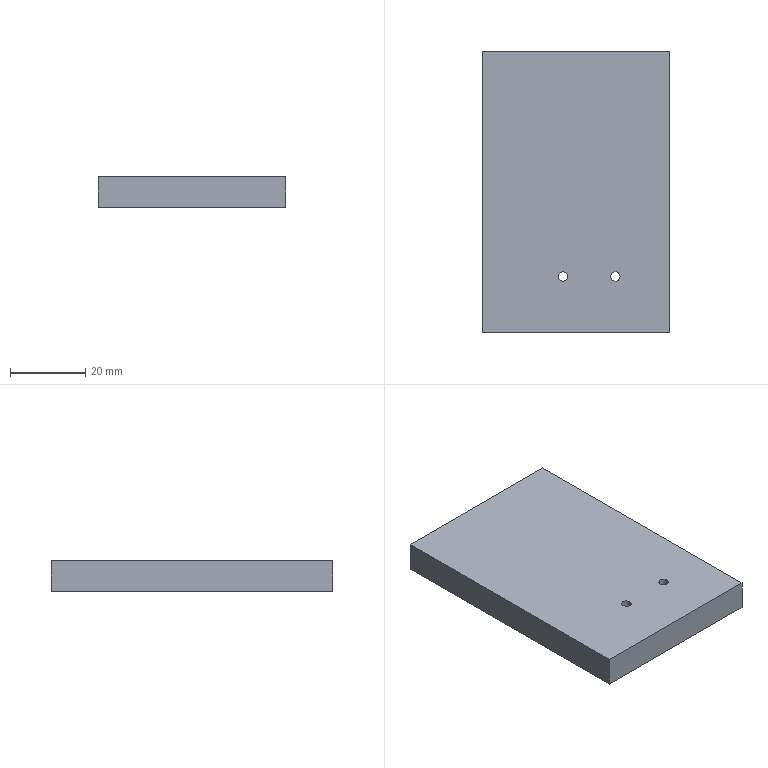Part | STEP file | GS mount plate | 1 solid | 16 faces | box 50 x 75 x 8 mm | volume 29332 mm3 | cylinder 8 | plane 8 | commonest cylinder face diameters 2.5 x4 5 x4
STEP:
#1=CARTESIAN_POINT('',(0.,0.,0.));
#2=DIRECTION('',(0.,0.,1.));
#3=DIRECTION('',(1.,0.,0.));
#4=AXIS2_PLACEMENT_3D('',#1,#2,#3);
#5=CARTESIAN_POINT('',(34.25,-60.,8.));
#6=VERTEX_POINT('',#5);
#7=CARTESIAN_POINT('',(34.25,-60.,0.));
#8=VERTEX_POINT('',#7);
#9=CARTESIAN_POINT('',(34.25,-60.,0.));
#10=DIRECTION('',(0.,0.,-1.));
#11=VECTOR('',#10,1.);
#12=LINE('',#9,#11);
#13=CARTESIAN_POINT('',(35.5,-60.,0.));
#14=DIRECTION('',(0.,0.,-1.));
#15=DIRECTION('',(-1.,0.,0.));
#16=AXIS2_PLACEMENT_3D('',#13,#14,#15);
#17=CYLINDRICAL_SURFACE('',#16,1.25);
#18=CARTESIAN_POINT('',(6.283,0.));
#19=DIRECTION('',(0.,1.));
#20=VECTOR('',#19,1.);
#21=LINE('',#18,#20);
#22=(GEOMETRIC_REPRESENTATION_CONTEXT(2)PARAMETRIC_REPRESENTATION_CONTEXT()REPRESENTATION_CONTEXT('',''));
#23=DEFINITIONAL_REPRESENTATION('',(#21),#22);
#24=PCURVE('',#17,#23);
#25=CARTESIAN_POINT('',(35.5,-60.,0.));
#26=DIRECTION('',(0.,0.,-1.));
#27=DIRECTION('',(-1.,0.,0.));
#28=AXIS2_PLACEMENT_3D('',#25,#26,#27);
#29=CYLINDRICAL_SURFACE('',#28,1.25);
#30=CARTESIAN_POINT('',(0.,0.));
#31=DIRECTION('',(0.,1.));
#32=VECTOR('',#31,1.);
#33=LINE('',#30,#32);
#34=(GEOMETRIC_REPRESENTATION_CONTEXT(2)PARAMETRIC_REPRESENTATION_CONTEXT()REPRESENTATION_CONTEXT('',''));
#35=DEFINITIONAL_REPRESENTATION('',(#33),#34);
#36=PCURVE('',#29,#35);
#37=SURFACE_CURVE('',#12,(#24,#36),.PCURVE_S1.);
#38=EDGE_CURVE('',#6,#8,#37,.T.);
#39=ORIENTED_EDGE('',*,*,#38,.T.);
#40=CARTESIAN_POINT('',(36.75,-60.,0.));
#41=VERTEX_POINT('',#40);
#42=CARTESIAN_POINT('',(35.5,-60.,0.));
#43=DIRECTION('',(0.,0.,-1.));
#44=DIRECTION('',(-1.,0.,0.));
#45=AXIS2_PLACEMENT_3D('',#42,#43,#44);
#46=CIRCLE('',#45,1.25);
#47=CARTESIAN_POINT('',(0.,0.));
#48=DIRECTION('',(1.,0.));
#49=VECTOR('',#48,1.);
#50=LINE('',#47,#49);
#51=(GEOMETRIC_REPRESENTATION_CONTEXT(2)PARAMETRIC_REPRESENTATION_CONTEXT()REPRESENTATION_CONTEXT('',''));
#52=DEFINITIONAL_REPRESENTATION('',(#50),#51);
#53=PCURVE('',#17,#52);
#54=CARTESIAN_POINT('',(0.,-75.,0.));
#55=DIRECTION('',(0.,0.,1.));
#56=DIRECTION('',(1.,0.,0.));
#57=AXIS2_PLACEMENT_3D('',#54,#55,#56);
#58=PLANE('',#57);
#59=CARTESIAN_POINT('',(34.25,15.));
#60=CARTESIAN_POINT('',(34.25,17.165));
#61=CARTESIAN_POINT('',(36.125,16.083));
#62=CARTESIAN_POINT('',(38.,15.));
#63=CARTESIAN_POINT('',(36.125,13.917));
#64=CARTESIAN_POINT('',(34.25,12.835));
#65=CARTESIAN_POINT('',(34.25,15.));
#66=(BOUNDED_CURVE()B_SPLINE_CURVE(2,(#59,#60,#61,#62,#63,#64,#65),.UNSPECIFIED.,.T.,.F.)B_SPLINE_CURVE_WITH_KNOTS((1,2,2,2,2,1),(-2.094,0.,2.094,4.189,6.283,8.378),.UNSPECIFIED.)CURVE()GEOMETRIC_REPRESENTATION_ITEM()RATIONAL_B_SPLINE_CURVE((1.,0.5,1.,0.5,1.,0.5,1.))REPRESENTATION_ITEM(''));
#67=(GEOMETRIC_REPRESENTATION_CONTEXT(2)PARAMETRIC_REPRESENTATION_CONTEXT()REPRESENTATION_CONTEXT('',''));
#68=DEFINITIONAL_REPRESENTATION('',(#66),#67);
#69=PCURVE('',#58,#68);
#70=SURFACE_CURVE('',#46,(#53,#69),.PCURVE_S1.);
#71=EDGE_CURVE('',#41,#8,#70,.T.);
#72=ORIENTED_EDGE('',*,*,#71,.F.);
#73=CARTESIAN_POINT('',(36.75,-60.,8.));
#74=VERTEX_POINT('',#73);
#75=CARTESIAN_POINT('',(36.75,-60.,0.));
#76=DIRECTION('',(0.,0.,-1.));
#77=VECTOR('',#76,1.);
#78=LINE('',#75,#77);
#79=CARTESIAN_POINT('',(3.142,0.));
#80=DIRECTION('',(0.,1.));
#81=VECTOR('',#80,1.);
#82=LINE('',#79,#81);
#83=(GEOMETRIC_REPRESENTATION_CONTEXT(2)PARAMETRIC_REPRESENTATION_CONTEXT()REPRESENTATION_CONTEXT('',''));
#84=DEFINITIONAL_REPRESENTATION('',(#82),#83);
#85=PCURVE('',#17,#84);
#86=CARTESIAN_POINT('',(3.142,0.));
#87=DIRECTION('',(0.,1.));
#88=VECTOR('',#87,1.);
#89=LINE('',#86,#88);
#90=(GEOMETRIC_REPRESENTATION_CONTEXT(2)PARAMETRIC_REPRESENTATION_CONTEXT()REPRESENTATION_CONTEXT('',''));
#91=DEFINITIONAL_REPRESENTATION('',(#89),#90);
#92=PCURVE('',#29,#91);
#93=SURFACE_CURVE('',#78,(#85,#92),.PCURVE_S1.);
#94=EDGE_CURVE('',#74,#41,#93,.T.);
#95=ORIENTED_EDGE('',*,*,#94,.F.);
#96=CARTESIAN_POINT('',(35.5,-60.,8.));
#97=DIRECTION('',(0.,0.,-1.));
#98=DIRECTION('',(-1.,0.,0.));
#99=AXIS2_PLACEMENT_3D('',#96,#97,#98);
#100=CIRCLE('',#99,1.25);
#101=CARTESIAN_POINT('',(0.,-8.));
#102=DIRECTION('',(1.,0.));
#103=VECTOR('',#102,1.);
#104=LINE('',#101,#103);
#105=(GEOMETRIC_REPRESENTATION_CONTEXT(2)PARAMETRIC_REPRESENTATION_CONTEXT()REPRESENTATION_CONTEXT('',''));
#106=DEFINITIONAL_REPRESENTATION('',(#104),#105);
#107=PCURVE('',#17,#106);
#108=CARTESIAN_POINT('',(0.,-75.,8.));
#109=DIRECTION('',(0.,0.,1.));
#110=DIRECTION('',(1.,0.,0.));
#111=AXIS2_PLACEMENT_3D('',#108,#109,#110);
#112=PLANE('',#111);
#113=CARTESIAN_POINT('',(34.25,15.));
#114=CARTESIAN_POINT('',(34.25,17.165));
#115=CARTESIAN_POINT('',(36.125,16.083));
#116=CARTESIAN_POINT('',(38.,15.));
#117=CARTESIAN_POINT('',(36.125,13.917));
#118=CARTESIAN_POINT('',(34.25,12.835));
#119=CARTESIAN_POINT('',(34.25,15.));
#120=(BOUNDED_CURVE()B_SPLINE_CURVE(2,(#113,#114,#115,#116,#117,#118,#119),.UNSPECIFIED.,.T.,.F.)B_SPLINE_CURVE_WITH_KNOTS((1,2,2,2,2,1),(-2.094,0.,2.094,4.189,6.283,8.378),.UNSPECIFIED.)CURVE()GEOMETRIC_REPRESENTATION_ITEM()RATIONAL_B_SPLINE_CURVE((1.,0.5,1.,0.5,1.,0.5,1.))REPRESENTATION_ITEM(''));
#121=(GEOMETRIC_REPRESENTATION_CONTEXT(2)PARAMETRIC_REPRESENTATION_CONTEXT()REPRESENTATION_CONTEXT('',''));
#122=DEFINITIONAL_REPRESENTATION('',(#120),#121);
#123=PCURVE('',#112,#122);
#124=SURFACE_CURVE('',#100,(#107,#123),.PCURVE_S1.);
#125=EDGE_CURVE('',#74,#6,#124,.T.);
#126=ORIENTED_EDGE('',*,*,#125,.T.);
#127=EDGE_LOOP('',(#39,#72,#95,#126));
#128=FACE_BOUND('',#127,.F.);
#129=ADVANCED_FACE('',(#128),#17,.F.);
#130=CARTESIAN_POINT('',(20.25,-60.,8.));
#131=VERTEX_POINT('',#130);
#132=CARTESIAN_POINT('',(20.25,-60.,0.));
#133=VERTEX_POINT('',#132);
#134=CARTESIAN_POINT('',(20.25,-60.,0.));
#135=DIRECTION('',(0.,0.,-1.));
#136=VECTOR('',#135,1.);
#137=LINE('',#134,#136);
#138=CARTESIAN_POINT('',(21.5,-60.,0.));
#139=DIRECTION('',(0.,0.,-1.));
#140=DIRECTION('',(-1.,0.,0.));
#141=AXIS2_PLACEMENT_3D('',#138,#139,#140);
#142=CYLINDRICAL_SURFACE('',#141,1.25);
#143=CARTESIAN_POINT('',(6.283,0.));
#144=DIRECTION('',(0.,1.));
#145=VECTOR('',#144,1.);
#146=LINE('',#143,#145);
#147=(GEOMETRIC_REPRESENTATION_CONTEXT(2)PARAMETRIC_REPRESENTATION_CONTEXT()REPRESENTATION_CONTEXT('',''));
#148=DEFINITIONAL_REPRESENTATION('',(#146),#147);
#149=PCURVE('',#142,#148);
#150=CARTESIAN_POINT('',(21.5,-60.,0.));
#151=DIRECTION('',(0.,0.,-1.));
#152=DIRECTION('',(-1.,0.,0.));
#153=AXIS2_PLACEMENT_3D('',#150,#151,#152);
#154=CYLINDRICAL_SURFACE('',#153,1.25);
#155=CARTESIAN_POINT('',(0.,0.));
#156=DIRECTION('',(0.,1.));
#157=VECTOR('',#156,1.);
#158=LINE('',#155,#157);
#159=(GEOMETRIC_REPRESENTATION_CONTEXT(2)PARAMETRIC_REPRESENTATION_CONTEXT()REPRESENTATION_CONTEXT('',''));
#160=DEFINITIONAL_REPRESENTATION('',(#158),#159);
#161=PCURVE('',#154,#160);
#162=SURFACE_CURVE('',#137,(#149,#161),.PCURVE_S1.);
#163=EDGE_CURVE('',#131,#133,#162,.T.);
#164=ORIENTED_EDGE('',*,*,#163,.T.);
#165=CARTESIAN_POINT('',(22.75,-60.,0.));
#166=VERTEX_POINT('',#165);
#167=CARTESIAN_POINT('',(21.5,-60.,0.));
#168=DIRECTION('',(0.,0.,-1.));
#169=DIRECTION('',(-1.,0.,0.));
#170=AXIS2_PLACEMENT_3D('',#167,#168,#169);
#171=CIRCLE('',#170,1.25);
#172=CARTESIAN_POINT('',(0.,0.));
#173=DIRECTION('',(1.,0.));
#174=VECTOR('',#173,1.);
#175=LINE('',#172,#174);
#176=(GEOMETRIC_REPRESENTATION_CONTEXT(2)PARAMETRIC_REPRESENTATION_CONTEXT()REPRESENTATION_CONTEXT('',''));
#177=DEFINITIONAL_REPRESENTATION('',(#175),#176);
#178=PCURVE('',#142,#177);
#179=CARTESIAN_POINT('',(20.25,15.));
#180=CARTESIAN_POINT('',(20.25,17.165));
#181=CARTESIAN_POINT('',(22.125,16.083));
#182=CARTESIAN_POINT('',(24.,15.));
#183=CARTESIAN_POINT('',(22.125,13.917));
#184=CARTESIAN_POINT('',(20.25,12.835));
#185=CARTESIAN_POINT('',(20.25,15.));
#186=(BOUNDED_CURVE()B_SPLINE_CURVE(2,(#179,#180,#181,#182,#183,#184,#185),.UNSPECIFIED.,.T.,.F.)B_SPLINE_CURVE_WITH_KNOTS((1,2,2,2,2,1),(-2.094,0.,2.094,4.189,6.283,8.378),.UNSPECIFIED.)CURVE()GEOMETRIC_REPRESENTATION_ITEM()RATIONAL_B_SPLINE_CURVE((1.,0.5,1.,0.5,1.,0.5,1.))REPRESENTATION_ITEM(''));
#187=(GEOMETRIC_REPRESENTATION_CONTEXT(2)PARAMETRIC_REPRESENTATION_CONTEXT()REPRESENTATION_CONTEXT('',''));
#188=DEFINITIONAL_REPRESENTATION('',(#186),#187);
#189=PCURVE('',#58,#188);
#190=SURFACE_CURVE('',#171,(#178,#189),.PCURVE_S1.);
#191=EDGE_CURVE('',#166,#133,#190,.T.);
#192=ORIENTED_EDGE('',*,*,#191,.F.);
#193=CARTESIAN_POINT('',(22.75,-60.,8.));
#194=VERTEX_POINT('',#193);
#195=CARTESIAN_POINT('',(22.75,-60.,0.));
#196=DIRECTION('',(0.,0.,-1.));
#197=VECTOR('',#196,1.);
#198=LINE('',#195,#197);
#199=CARTESIAN_POINT('',(3.142,0.));
#200=DIRECTION('',(0.,1.));
#201=VECTOR('',#200,1.);
#202=LINE('',#199,#201);
#203=(GEOMETRIC_REPRESENTATION_CONTEXT(2)PARAMETRIC_REPRESENTATION_CONTEXT()REPRESENTATION_CONTEXT('',''));
#204=DEFINITIONAL_REPRESENTATION('',(#202),#203);
#205=PCURVE('',#142,#204);
#206=CARTESIAN_POINT('',(3.142,0.));
#207=DIRECTION('',(0.,1.));
#208=VECTOR('',#207,1.);
#209=LINE('',#206,#208);
#210=(GEOMETRIC_REPRESENTATION_CONTEXT(2)PARAMETRIC_REPRESENTATION_CONTEXT()REPRESENTATION_CONTEXT('',''));
#211=DEFINITIONAL_REPRESENTATION('',(#209),#210);
#212=PCURVE('',#154,#211);
#213=SURFACE_CURVE('',#198,(#205,#212),.PCURVE_S1.);
#214=EDGE_CURVE('',#194,#166,#213,.T.);
#215=ORIENTED_EDGE('',*,*,#214,.F.);
#216=CARTESIAN_POINT('',(21.5,-60.,8.));
#217=DIRECTION('',(0.,0.,-1.));
#218=DIRECTION('',(-1.,0.,0.));
#219=AXIS2_PLACEMENT_3D('',#216,#217,#218);
#220=CIRCLE('',#219,1.25);
#221=CARTESIAN_POINT('',(0.,-8.));
#222=DIRECTION('',(1.,0.));
#223=VECTOR('',#222,1.);
#224=LINE('',#221,#223);
#225=(GEOMETRIC_REPRESENTATION_CONTEXT(2)PARAMETRIC_REPRESENTATION_CONTEXT()REPRESENTATION_CONTEXT('',''));
#226=DEFINITIONAL_REPRESENTATION('',(#224),#225);
#227=PCURVE('',#142,#226);
#228=CARTESIAN_POINT('',(20.25,15.));
#229=CARTESIAN_POINT('',(20.25,17.165));
#230=CARTESIAN_POINT('',(22.125,16.083));
#231=CARTESIAN_POINT('',(24.,15.));
#232=CARTESIAN_POINT('',(22.125,13.917));
#233=CARTESIAN_POINT('',(20.25,12.835));
#234=CARTESIAN_POINT('',(20.25,15.));
#235=(BOUNDED_CURVE()B_SPLINE_CURVE(2,(#228,#229,#230,#231,#232,#233,#234),.UNSPECIFIED.,.T.,.F.)B_SPLINE_CURVE_WITH_KNOTS((1,2,2,2,2,1),(-2.094,0.,2.094,4.189,6.283,8.378),.UNSPECIFIED.)CURVE()GEOMETRIC_REPRESENTATION_ITEM()RATIONAL_B_SPLINE_CURVE((1.,0.5,1.,0.5,1.,0.5,1.))REPRESENTATION_ITEM(''));
#236=(GEOMETRIC_REPRESENTATION_CONTEXT(2)PARAMETRIC_REPRESENTATION_CONTEXT()REPRESENTATION_CONTEXT('',''));
#237=DEFINITIONAL_REPRESENTATION('',(#235),#236);
#238=PCURVE('',#112,#237);
#239=SURFACE_CURVE('',#220,(#227,#238),.PCURVE_S1.);
#240=EDGE_CURVE('',#194,#131,#239,.T.);
#241=ORIENTED_EDGE('',*,*,#240,.T.);
#242=EDGE_LOOP('',(#164,#192,#215,#241));
#243=FACE_BOUND('',#242,.F.);
#244=ADVANCED_FACE('',(#243),#142,.F.);
#245=CARTESIAN_POINT('',(43.,-15.,6.5));
#246=VERTEX_POINT('',#245);
#247=CARTESIAN_POINT('',(43.,0.,6.5));
#248=VERTEX_POINT('',#247);
#249=CARTESIAN_POINT('',(43.,0.,6.5));
#250=DIRECTION('',(0.,1.,0.));
#251=VECTOR('',#250,1.);
#252=LINE('',#249,#251);
#253=CARTESIAN_POINT('',(43.,0.,4.));
#254=DIRECTION('',(0.,1.,0.));
#255=DIRECTION('',(0.,0.,1.));
#256=AXIS2_PLACEMENT_3D('',#253,#254,#255);
#257=CYLINDRICAL_SURFACE('',#256,2.5);
#258=CARTESIAN_POINT('',(6.283,0.));
#259=DIRECTION('',(0.,1.));
#260=VECTOR('',#259,1.);
#261=LINE('',#258,#260);
#262=(GEOMETRIC_REPRESENTATION_CONTEXT(2)PARAMETRIC_REPRESENTATION_CONTEXT()REPRESENTATION_CONTEXT('',''));
#263=DEFINITIONAL_REPRESENTATION('',(#261),#262);
#264=PCURVE('',#257,#263);
#265=CARTESIAN_POINT('',(43.,0.,4.));
#266=DIRECTION('',(0.,1.,0.));
#267=DIRECTION('',(0.,0.,1.));
#268=AXIS2_PLACEMENT_3D('',#265,#266,#267);
#269=CYLINDRICAL_SURFACE('',#268,2.5);
#270=CARTESIAN_POINT('',(0.,0.));
#271=DIRECTION('',(0.,1.));
#272=VECTOR('',#271,1.);
#273=LINE('',#270,#272);
#274=(GEOMETRIC_REPRESENTATION_CONTEXT(2)PARAMETRIC_REPRESENTATION_CONTEXT()REPRESENTATION_CONTEXT('',''));
#275=DEFINITIONAL_REPRESENTATION('',(#273),#274);
#276=PCURVE('',#269,#275);
#277=SURFACE_CURVE('',#252,(#264,#276),.PCURVE_S1.);
#278=EDGE_CURVE('',#246,#248,#277,.T.);
#279=ORIENTED_EDGE('',*,*,#278,.T.);
#280=CARTESIAN_POINT('',(43.,0.,1.5));
#281=VERTEX_POINT('',#280);
#282=CARTESIAN_POINT('',(43.,0.,4.));
#283=DIRECTION('',(0.,1.,0.));
#284=DIRECTION('',(0.,0.,1.));
#285=AXIS2_PLACEMENT_3D('',#282,#283,#284);
#286=CIRCLE('',#285,2.5);
#287=CARTESIAN_POINT('',(0.,0.));
#288=DIRECTION('',(1.,0.));
#289=VECTOR('',#288,1.);
#290=LINE('',#287,#289);
#291=(GEOMETRIC_REPRESENTATION_CONTEXT(2)PARAMETRIC_REPRESENTATION_CONTEXT()REPRESENTATION_CONTEXT('',''));
#292=DEFINITIONAL_REPRESENTATION('',(#290),#291);
#293=PCURVE('',#257,#292);
#294=CARTESIAN_POINT('',(0.,0.,8.));
#295=DIRECTION('',(0.,-1.,0.));
#296=DIRECTION('',(0.,0.,-1.));
#297=AXIS2_PLACEMENT_3D('',#294,#295,#296);
#298=PLANE('',#297);
#299=CARTESIAN_POINT('',(1.5,43.));
#300=CARTESIAN_POINT('',(1.5,47.33));
#301=CARTESIAN_POINT('',(5.25,45.165));
#302=CARTESIAN_POINT('',(9.,43.));
#303=CARTESIAN_POINT('',(5.25,40.835));
#304=CARTESIAN_POINT('',(1.5,38.67));
#305=CARTESIAN_POINT('',(1.5,43.));
#306=(BOUNDED_CURVE()B_SPLINE_CURVE(2,(#299,#300,#301,#302,#303,#304,#305),.UNSPECIFIED.,.T.,.F.)B_SPLINE_CURVE_WITH_KNOTS((1,2,2,2,2,1),(-2.094,0.,2.094,4.189,6.283,8.378),.UNSPECIFIED.)CURVE()GEOMETRIC_REPRESENTATION_ITEM()RATIONAL_B_SPLINE_CURVE((1.,0.5,1.,0.5,1.,0.5,1.))REPRESENTATION_ITEM(''));
#307=(GEOMETRIC_REPRESENTATION_CONTEXT(2)PARAMETRIC_REPRESENTATION_CONTEXT()REPRESENTATION_CONTEXT('',''));
#308=DEFINITIONAL_REPRESENTATION('',(#306),#307);
#309=PCURVE('',#298,#308);
#310=SURFACE_CURVE('',#286,(#293,#309),.PCURVE_S1.);
#311=EDGE_CURVE('',#281,#248,#310,.T.);
#312=ORIENTED_EDGE('',*,*,#311,.F.);
#313=CARTESIAN_POINT('',(43.,-15.,1.5));
#314=VERTEX_POINT('',#313);
#315=CARTESIAN_POINT('',(43.,0.,1.5));
#316=DIRECTION('',(0.,1.,0.));
#317=VECTOR('',#316,1.);
#318=LINE('',#315,#317);
#319=CARTESIAN_POINT('',(3.142,0.));
#320=DIRECTION('',(0.,1.));
#321=VECTOR('',#320,1.);
#322=LINE('',#319,#321);
#323=(GEOMETRIC_REPRESENTATION_CONTEXT(2)PARAMETRIC_REPRESENTATION_CONTEXT()REPRESENTATION_CONTEXT('',''));
#324=DEFINITIONAL_REPRESENTATION('',(#322),#323);
#325=PCURVE('',#257,#324);
#326=CARTESIAN_POINT('',(3.142,0.));
#327=DIRECTION('',(0.,1.));
#328=VECTOR('',#327,1.);
#329=LINE('',#326,#328);
#330=(GEOMETRIC_REPRESENTATION_CONTEXT(2)PARAMETRIC_REPRESENTATION_CONTEXT()REPRESENTATION_CONTEXT('',''));
#331=DEFINITIONAL_REPRESENTATION('',(#329),#330);
#332=PCURVE('',#269,#331);
#333=SURFACE_CURVE('',#318,(#325,#332),.PCURVE_S1.);
#334=EDGE_CURVE('',#314,#281,#333,.T.);
#335=ORIENTED_EDGE('',*,*,#334,.F.);
#336=CARTESIAN_POINT('',(43.,-15.,4.));
#337=DIRECTION('',(0.,1.,0.));
#338=DIRECTION('',(0.,0.,1.));
#339=AXIS2_PLACEMENT_3D('',#336,#337,#338);
#340=CIRCLE('',#339,2.5);
#341=CARTESIAN_POINT('',(0.,-15.));
#342=DIRECTION('',(1.,0.));
#343=VECTOR('',#342,1.);
#344=LINE('',#341,#343);
#345=(GEOMETRIC_REPRESENTATION_CONTEXT(2)PARAMETRIC_REPRESENTATION_CONTEXT()REPRESENTATION_CONTEXT('',''));
#346=DEFINITIONAL_REPRESENTATION('',(#344),#345);
#347=PCURVE('',#257,#346);
#348=CARTESIAN_POINT('',(43.,-15.,4.));
#349=DIRECTION('',(0.,-1.,0.));
#350=DIRECTION('',(0.,0.,-1.));
#351=AXIS2_PLACEMENT_3D('',#348,#349,#350);
#352=PLANE('',#351);
#353=CARTESIAN_POINT('',(-2.5,0.));
#354=CARTESIAN_POINT('',(-2.5,4.33));
#355=CARTESIAN_POINT('',(1.25,2.165));
#356=CARTESIAN_POINT('',(5.,0.));
#357=CARTESIAN_POINT('',(1.25,-2.165));
#358=CARTESIAN_POINT('',(-2.5,-4.33));
#359=CARTESIAN_POINT('',(-2.5,0.));
#360=(BOUNDED_CURVE()B_SPLINE_CURVE(2,(#353,#354,#355,#356,#357,#358,#359),.UNSPECIFIED.,.T.,.F.)B_SPLINE_CURVE_WITH_KNOTS((1,2,2,2,2,1),(-2.094,0.,2.094,4.189,6.283,8.378),.UNSPECIFIED.)CURVE()GEOMETRIC_REPRESENTATION_ITEM()RATIONAL_B_SPLINE_CURVE((1.,0.5,1.,0.5,1.,0.5,1.))REPRESENTATION_ITEM(''));
#361=(GEOMETRIC_REPRESENTATION_CONTEXT(2)PARAMETRIC_REPRESENTATION_CONTEXT()REPRESENTATION_CONTEXT('',''));
#362=DEFINITIONAL_REPRESENTATION('',(#360),#361);
#363=PCURVE('',#352,#362);
#364=SURFACE_CURVE('',#340,(#347,#363),.PCURVE_S1.);
#365=EDGE_CURVE('',#314,#246,#364,.T.);
#366=ORIENTED_EDGE('',*,*,#365,.T.);
#367=EDGE_LOOP('',(#279,#312,#335,#366));
#368=FACE_BOUND('',#367,.F.);
#369=ADVANCED_FACE('',(#368),#257,.F.);
#370=CARTESIAN_POINT('',(7.,-15.,6.5));
#371=VERTEX_POINT('',#370);
#372=CARTESIAN_POINT('',(7.,0.,6.5));
#373=VERTEX_POINT('',#372);
#374=CARTESIAN_POINT('',(7.,0.,6.5));
#375=DIRECTION('',(0.,1.,0.));
#376=VECTOR('',#375,1.);
#377=LINE('',#374,#376);
#378=CARTESIAN_POINT('',(7.,0.,4.));
#379=DIRECTION('',(0.,1.,0.));
#380=DIRECTION('',(0.,0.,1.));
#381=AXIS2_PLACEMENT_3D('',#378,#379,#380);
#382=CYLINDRICAL_SURFACE('',#381,2.5);
#383=CARTESIAN_POINT('',(6.283,0.));
#384=DIRECTION('',(0.,1.));
#385=VECTOR('',#384,1.);
#386=LINE('',#383,#385);
#387=(GEOMETRIC_REPRESENTATION_CONTEXT(2)PARAMETRIC_REPRESENTATION_CONTEXT()REPRESENTATION_CONTEXT('',''));
#388=DEFINITIONAL_REPRESENTATION('',(#386),#387);
#389=PCURVE('',#382,#388);
#390=CARTESIAN_POINT('',(7.,0.,4.));
#391=DIRECTION('',(0.,1.,0.));
#392=DIRECTION('',(0.,0.,1.));
#393=AXIS2_PLACEMENT_3D('',#390,#391,#392);
#394=CYLINDRICAL_SURFACE('',#393,2.5);
#395=CARTESIAN_POINT('',(0.,0.));
#396=DIRECTION('',(0.,1.));
#397=VECTOR('',#396,1.);
#398=LINE('',#395,#397);
#399=(GEOMETRIC_REPRESENTATION_CONTEXT(2)PARAMETRIC_REPRESENTATION_CONTEXT()REPRESENTATION_CONTEXT('',''));
#400=DEFINITIONAL_REPRESENTATION('',(#398),#399);
#401=PCURVE('',#394,#400);
#402=SURFACE_CURVE('',#377,(#389,#401),.PCURVE_S1.);
#403=EDGE_CURVE('',#371,#373,#402,.T.);
#404=ORIENTED_EDGE('',*,*,#403,.T.);
#405=CARTESIAN_POINT('',(7.,0.,1.5));
#406=VERTEX_POINT('',#405);
#407=CARTESIAN_POINT('',(7.,0.,4.));
#408=DIRECTION('',(0.,1.,0.));
#409=DIRECTION('',(0.,0.,1.));
#410=AXIS2_PLACEMENT_3D('',#407,#408,#409);
#411=CIRCLE('',#410,2.5);
#412=CARTESIAN_POINT('',(0.,0.));
#413=DIRECTION('',(1.,0.));
#414=VECTOR('',#413,1.);
#415=LINE('',#412,#414);
#416=(GEOMETRIC_REPRESENTATION_CONTEXT(2)PARAMETRIC_REPRESENTATION_CONTEXT()REPRESENTATION_CONTEXT('',''));
#417=DEFINITIONAL_REPRESENTATION('',(#415),#416);
#418=PCURVE('',#382,#417);
#419=CARTESIAN_POINT('',(1.5,7.));
#420=CARTESIAN_POINT('',(1.5,11.33));
#421=CARTESIAN_POINT('',(5.25,9.165));
#422=CARTESIAN_POINT('',(9.,7.));
#423=CARTESIAN_POINT('',(5.25,4.835));
#424=CARTESIAN_POINT('',(1.5,2.67));
#425=CARTESIAN_POINT('',(1.5,7.));
#426=(BOUNDED_CURVE()B_SPLINE_CURVE(2,(#419,#420,#421,#422,#423,#424,#425),.UNSPECIFIED.,.T.,.F.)B_SPLINE_CURVE_WITH_KNOTS((1,2,2,2,2,1),(-2.094,0.,2.094,4.189,6.283,8.378),.UNSPECIFIED.)CURVE()GEOMETRIC_REPRESENTATION_ITEM()RATIONAL_B_SPLINE_CURVE((1.,0.5,1.,0.5,1.,0.5,1.))REPRESENTATION_ITEM(''));
#427=(GEOMETRIC_REPRESENTATION_CONTEXT(2)PARAMETRIC_REPRESENTATION_CONTEXT()REPRESENTATION_CONTEXT('',''));
#428=DEFINITIONAL_REPRESENTATION('',(#426),#427);
#429=PCURVE('',#298,#428);
#430=SURFACE_CURVE('',#411,(#418,#429),.PCURVE_S1.);
#431=EDGE_CURVE('',#406,#373,#430,.T.);
#432=ORIENTED_EDGE('',*,*,#431,.F.);
#433=CARTESIAN_POINT('',(7.,-15.,1.5));
#434=VERTEX_POINT('',#433);
#435=CARTESIAN_POINT('',(7.,0.,1.5));
#436=DIRECTION('',(0.,1.,0.));
#437=VECTOR('',#436,1.);
#438=LINE('',#435,#437);
#439=CARTESIAN_POINT('',(3.142,0.));
#440=DIRECTION('',(0.,1.));
#441=VECTOR('',#440,1.);
#442=LINE('',#439,#441);
#443=(GEOMETRIC_REPRESENTATION_CONTEXT(2)PARAMETRIC_REPRESENTATION_CONTEXT()REPRESENTATION_CONTEXT('',''));
#444=DEFINITIONAL_REPRESENTATION('',(#442),#443);
#445=PCURVE('',#382,#444);
#446=CARTESIAN_POINT('',(3.142,0.));
#447=DIRECTION('',(0.,1.));
#448=VECTOR('',#447,1.);
#449=LINE('',#446,#448);
#450=(GEOMETRIC_REPRESENTATION_CONTEXT(2)PARAMETRIC_REPRESENTATION_CONTEXT()REPRESENTATION_CONTEXT('',''));
#451=DEFINITIONAL_REPRESENTATION('',(#449),#450);
#452=PCURVE('',#394,#451);
#453=SURFACE_CURVE('',#438,(#445,#452),.PCURVE_S1.);
#454=EDGE_CURVE('',#434,#406,#453,.T.);
#455=ORIENTED_EDGE('',*,*,#454,.F.);
#456=CARTESIAN_POINT('',(7.,-15.,4.));
#457=DIRECTION('',(0.,1.,0.));
#458=DIRECTION('',(0.,0.,1.));
#459=AXIS2_PLACEMENT_3D('',#456,#457,#458);
#460=CIRCLE('',#459,2.5);
#461=CARTESIAN_POINT('',(0.,-15.));
#462=DIRECTION('',(1.,0.));
#463=VECTOR('',#462,1.);
#464=LINE('',#461,#463);
#465=(GEOMETRIC_REPRESENTATION_CONTEXT(2)PARAMETRIC_REPRESENTATION_CONTEXT()REPRESENTATION_CONTEXT('',''));
#466=DEFINITIONAL_REPRESENTATION('',(#464),#465);
#467=PCURVE('',#382,#466);
#468=CARTESIAN_POINT('',(7.,-15.,4.));
#469=DIRECTION('',(0.,-1.,0.));
#470=DIRECTION('',(0.,0.,-1.));
#471=AXIS2_PLACEMENT_3D('',#468,#469,#470);
#472=PLANE('',#471);
#473=CARTESIAN_POINT('',(-2.5,0.));
#474=CARTESIAN_POINT('',(-2.5,4.33));
#475=CARTESIAN_POINT('',(1.25,2.165));
#476=CARTESIAN_POINT('',(5.,0.));
#477=CARTESIAN_POINT('',(1.25,-2.165));
#478=CARTESIAN_POINT('',(-2.5,-4.33));
#479=CARTESIAN_POINT('',(-2.5,0.));
#480=(BOUNDED_CURVE()B_SPLINE_CURVE(2,(#473,#474,#475,#476,#477,#478,#479),.UNSPECIFIED.,.T.,.F.)B_SPLINE_CURVE_WITH_KNOTS((1,2,2,2,2,1),(-2.094,0.,2.094,4.189,6.283,8.378),.UNSPECIFIED.)CURVE()GEOMETRIC_REPRESENTATION_ITEM()RATIONAL_B_SPLINE_CURVE((1.,0.5,1.,0.5,1.,0.5,1.))REPRESENTATION_ITEM(''));
#481=(GEOMETRIC_REPRESENTATION_CONTEXT(2)PARAMETRIC_REPRESENTATION_CONTEXT()REPRESENTATION_CONTEXT('',''));
#482=DEFINITIONAL_REPRESENTATION('',(#480),#481);
#483=PCURVE('',#472,#482);
#484=SURFACE_CURVE('',#460,(#467,#483),.PCURVE_S1.);
#485=EDGE_CURVE('',#434,#371,#484,.T.);
#486=ORIENTED_EDGE('',*,*,#485,.T.);
#487=EDGE_LOOP('',(#404,#432,#455,#486));
#488=FACE_BOUND('',#487,.F.);
#489=ADVANCED_FACE('',(#488),#382,.F.);
#490=CARTESIAN_POINT('',(50.,0.,0.));
#491=VERTEX_POINT('',#490);
#492=CARTESIAN_POINT('',(0.,0.,0.));
#493=VERTEX_POINT('',#492);
#494=CARTESIAN_POINT('',(0.,0.,0.));
#495=DIRECTION('',(-1.,0.,0.));
#496=VECTOR('',#495,1.);
#497=LINE('',#494,#496);
#498=CARTESIAN_POINT('',(0.,75.));
#499=DIRECTION('',(-1.,0.));
#500=VECTOR('',#499,1.);
#501=LINE('',#498,#500);
#502=(GEOMETRIC_REPRESENTATION_CONTEXT(2)PARAMETRIC_REPRESENTATION_CONTEXT()REPRESENTATION_CONTEXT('',''));
#503=DEFINITIONAL_REPRESENTATION('',(#501),#502);
#504=PCURVE('',#58,#503);
#505=CARTESIAN_POINT('',(8.,0.));
#506=DIRECTION('',(0.,-1.));
#507=VECTOR('',#506,1.);
#508=LINE('',#505,#507);
#509=(GEOMETRIC_REPRESENTATION_CONTEXT(2)PARAMETRIC_REPRESENTATION_CONTEXT()REPRESENTATION_CONTEXT('',''));
#510=DEFINITIONAL_REPRESENTATION('',(#508),#509);
#511=PCURVE('',#298,#510);
#512=SURFACE_CURVE('',#497,(#504,#511),.PCURVE_S1.);
#513=EDGE_CURVE('',#491,#493,#512,.T.);
#514=ORIENTED_EDGE('',*,*,#513,.F.);
#515=CARTESIAN_POINT('',(50.,-75.,0.));
#516=VERTEX_POINT('',#515);
#517=CARTESIAN_POINT('',(50.,-75.,0.));
#518=DIRECTION('',(0.,1.,0.));
#519=VECTOR('',#518,1.);
#520=LINE('',#517,#519);
#521=CARTESIAN_POINT('',(50.,0.));
#522=DIRECTION('',(0.,1.));
#523=VECTOR('',#522,1.);
#524=LINE('',#521,#523);
#525=(GEOMETRIC_REPRESENTATION_CONTEXT(2)PARAMETRIC_REPRESENTATION_CONTEXT()REPRESENTATION_CONTEXT('',''));
#526=DEFINITIONAL_REPRESENTATION('',(#524),#525);
#527=PCURVE('',#58,#526);
#528=CARTESIAN_POINT('',(50.,0.,8.));
#529=DIRECTION('',(-1.,0.,0.));
#530=DIRECTION('',(0.,-1.,0.));
#531=AXIS2_PLACEMENT_3D('',#528,#529,#530);
#532=PLANE('',#531);
#533=CARTESIAN_POINT('',(75.,-8.));
#534=DIRECTION('',(-1.,0.));
#535=VECTOR('',#534,1.);
#536=LINE('',#533,#535);
#537=(GEOMETRIC_REPRESENTATION_CONTEXT(2)PARAMETRIC_REPRESENTATION_CONTEXT()REPRESENTATION_CONTEXT('',''));
#538=DEFINITIONAL_REPRESENTATION('',(#536),#537);
#539=PCURVE('',#532,#538);
#540=SURFACE_CURVE('',#520,(#527,#539),.PCURVE_S1.);
#541=EDGE_CURVE('',#516,#491,#540,.T.);
#542=ORIENTED_EDGE('',*,*,#541,.F.);
#543=CARTESIAN_POINT('',(0.,-75.,0.));
#544=VERTEX_POINT('',#543);
#545=CARTESIAN_POINT('',(0.,-75.,0.));
#546=DIRECTION('',(1.,0.,0.));
#547=VECTOR('',#546,1.);
#548=LINE('',#545,#547);
#549=CARTESIAN_POINT('',(0.,0.));
#550=DIRECTION('',(1.,0.));
#551=VECTOR('',#550,1.);
#552=LINE('',#549,#551);
#553=(GEOMETRIC_REPRESENTATION_CONTEXT(2)PARAMETRIC_REPRESENTATION_CONTEXT()REPRESENTATION_CONTEXT('',''));
#554=DEFINITIONAL_REPRESENTATION('',(#552),#553);
#555=PCURVE('',#58,#554);
#556=CARTESIAN_POINT('',(0.,-75.,8.));
#557=DIRECTION('',(0.,1.,0.));
#558=DIRECTION('',(0.,0.,1.));
#559=AXIS2_PLACEMENT_3D('',#556,#557,#558);
#560=PLANE('',#559);
#561=CARTESIAN_POINT('',(-8.,0.));
#562=DIRECTION('',(0.,1.));
#563=VECTOR('',#562,1.);
#564=LINE('',#561,#563);
#565=(GEOMETRIC_REPRESENTATION_CONTEXT(2)PARAMETRIC_REPRESENTATION_CONTEXT()REPRESENTATION_CONTEXT('',''));
#566=DEFINITIONAL_REPRESENTATION('',(#564),#565);
#567=PCURVE('',#560,#566);
#568=SURFACE_CURVE('',#548,(#555,#567),.PCURVE_S1.);
#569=EDGE_CURVE('',#544,#516,#568,.T.);
#570=ORIENTED_EDGE('',*,*,#569,.F.);
#571=CARTESIAN_POINT('',(0.,-75.,0.));
#572=DIRECTION('',(0.,-1.,0.));
#573=VECTOR('',#572,1.);
#574=LINE('',#571,#573);
#575=CARTESIAN_POINT('',(0.,0.));
#576=DIRECTION('',(0.,-1.));
#577=VECTOR('',#576,1.);
#578=LINE('',#575,#577);
#579=(GEOMETRIC_REPRESENTATION_CONTEXT(2)PARAMETRIC_REPRESENTATION_CONTEXT()REPRESENTATION_CONTEXT('',''));
#580=DEFINITIONAL_REPRESENTATION('',(#578),#579);
#581=PCURVE('',#58,#580);
#582=CARTESIAN_POINT('',(0.,0.,8.));
#583=DIRECTION('',(1.,0.,0.));
#584=DIRECTION('',(0.,1.,0.));
#585=AXIS2_PLACEMENT_3D('',#582,#583,#584);
#586=PLANE('',#585);
#587=CARTESIAN_POINT('',(-75.,-8.));
#588=DIRECTION('',(-1.,0.));
#589=VECTOR('',#588,1.);
#590=LINE('',#587,#589);
#591=(GEOMETRIC_REPRESENTATION_CONTEXT(2)PARAMETRIC_REPRESENTATION_CONTEXT()REPRESENTATION_CONTEXT('',''));
#592=DEFINITIONAL_REPRESENTATION('',(#590),#591);
#593=PCURVE('',#586,#592);
#594=SURFACE_CURVE('',#574,(#581,#593),.PCURVE_S1.);
#595=EDGE_CURVE('',#493,#544,#594,.T.);
#596=ORIENTED_EDGE('',*,*,#595,.F.);
#597=EDGE_LOOP('',(#514,#542,#570,#596));
#598=FACE_BOUND('',#597,.T.);
#599=CARTESIAN_POINT('',(35.5,-60.,0.));
#600=DIRECTION('',(0.,0.,-1.));
#601=DIRECTION('',(-1.,0.,0.));
#602=AXIS2_PLACEMENT_3D('',#599,#600,#601);
#603=CIRCLE('',#602,1.25);
#604=CARTESIAN_POINT('',(34.25,15.));
#605=CARTESIAN_POINT('',(34.25,17.165));
#606=CARTESIAN_POINT('',(36.125,16.083));
#607=CARTESIAN_POINT('',(38.,15.));
#608=CARTESIAN_POINT('',(36.125,13.917));
#609=CARTESIAN_POINT('',(34.25,12.835));
#610=CARTESIAN_POINT('',(34.25,15.));
#611=(BOUNDED_CURVE()B_SPLINE_CURVE(2,(#604,#605,#606,#607,#608,#609,#610),.UNSPECIFIED.,.T.,.F.)B_SPLINE_CURVE_WITH_KNOTS((1,2,2,2,2,1),(-2.094,0.,2.094,4.189,6.283,8.378),.UNSPECIFIED.)CURVE()GEOMETRIC_REPRESENTATION_ITEM()RATIONAL_B_SPLINE_CURVE((1.,0.5,1.,0.5,1.,0.5,1.))REPRESENTATION_ITEM(''));
#612=(GEOMETRIC_REPRESENTATION_CONTEXT(2)PARAMETRIC_REPRESENTATION_CONTEXT()REPRESENTATION_CONTEXT('',''));
#613=DEFINITIONAL_REPRESENTATION('',(#611),#612);
#614=PCURVE('',#58,#613);
#615=CARTESIAN_POINT('',(0.,0.));
#616=DIRECTION('',(1.,0.));
#617=VECTOR('',#616,1.);
#618=LINE('',#615,#617);
#619=(GEOMETRIC_REPRESENTATION_CONTEXT(2)PARAMETRIC_REPRESENTATION_CONTEXT()REPRESENTATION_CONTEXT('',''));
#620=DEFINITIONAL_REPRESENTATION('',(#618),#619);
#621=PCURVE('',#29,#620);
#622=SURFACE_CURVE('',#603,(#614,#621),.PCURVE_S1.);
#623=EDGE_CURVE('',#8,#41,#622,.T.);
#624=ORIENTED_EDGE('',*,*,#623,.F.);
#625=ORIENTED_EDGE('',*,*,#71,.F.);
#626=EDGE_LOOP('',(#624,#625));
#627=FACE_BOUND('',#626,.T.);
#628=CARTESIAN_POINT('',(21.5,-60.,0.));
#629=DIRECTION('',(0.,0.,-1.));
#630=DIRECTION('',(-1.,0.,0.));
#631=AXIS2_PLACEMENT_3D('',#628,#629,#630);
#632=CIRCLE('',#631,1.25);
#633=CARTESIAN_POINT('',(20.25,15.));
#634=CARTESIAN_POINT('',(20.25,17.165));
#635=CARTESIAN_POINT('',(22.125,16.083));
#636=CARTESIAN_POINT('',(24.,15.));
#637=CARTESIAN_POINT('',(22.125,13.917));
#638=CARTESIAN_POINT('',(20.25,12.835));
#639=CARTESIAN_POINT('',(20.25,15.));
#640=(BOUNDED_CURVE()B_SPLINE_CURVE(2,(#633,#634,#635,#636,#637,#638,#639),.UNSPECIFIED.,.T.,.F.)B_SPLINE_CURVE_WITH_KNOTS((1,2,2,2,2,1),(-2.094,0.,2.094,4.189,6.283,8.378),.UNSPECIFIED.)CURVE()GEOMETRIC_REPRESENTATION_ITEM()RATIONAL_B_SPLINE_CURVE((1.,0.5,1.,0.5,1.,0.5,1.))REPRESENTATION_ITEM(''));
#641=(GEOMETRIC_REPRESENTATION_CONTEXT(2)PARAMETRIC_REPRESENTATION_CONTEXT()REPRESENTATION_CONTEXT('',''));
#642=DEFINITIONAL_REPRESENTATION('',(#640),#641);
#643=PCURVE('',#58,#642);
#644=CARTESIAN_POINT('',(0.,0.));
#645=DIRECTION('',(1.,0.));
#646=VECTOR('',#645,1.);
#647=LINE('',#644,#646);
#648=(GEOMETRIC_REPRESENTATION_CONTEXT(2)PARAMETRIC_REPRESENTATION_CONTEXT()REPRESENTATION_CONTEXT('',''));
#649=DEFINITIONAL_REPRESENTATION('',(#647),#648);
#650=PCURVE('',#154,#649);
#651=SURFACE_CURVE('',#632,(#643,#650),.PCURVE_S1.);
#652=EDGE_CURVE('',#133,#166,#651,.T.);
#653=ORIENTED_EDGE('',*,*,#652,.F.);
#654=ORIENTED_EDGE('',*,*,#191,.F.);
#655=EDGE_LOOP('',(#653,#654));
#656=FACE_BOUND('',#655,.T.);
#657=ADVANCED_FACE('',(#598,#627,#656),#58,.F.);
#658=CARTESIAN_POINT('',(0.,-75.,8.));
#659=VERTEX_POINT('',#658);
#660=CARTESIAN_POINT('',(0.,-75.,8.));
#661=DIRECTION('',(0.,0.,-1.));
#662=VECTOR('',#661,1.);
#663=LINE('',#660,#662);
#664=CARTESIAN_POINT('',(-75.,0.));
#665=DIRECTION('',(0.,-1.));
#666=VECTOR('',#665,1.);
#667=LINE('',#664,#666);
#668=(GEOMETRIC_REPRESENTATION_CONTEXT(2)PARAMETRIC_REPRESENTATION_CONTEXT()REPRESENTATION_CONTEXT('',''));
#669=DEFINITIONAL_REPRESENTATION('',(#667),#668);
#670=PCURVE('',#586,#669);
#671=CARTESIAN_POINT('',(0.,0.));
#672=DIRECTION('',(-1.,0.));
#673=VECTOR('',#672,1.);
#674=LINE('',#671,#673);
#675=(GEOMETRIC_REPRESENTATION_CONTEXT(2)PARAMETRIC_REPRESENTATION_CONTEXT()REPRESENTATION_CONTEXT('',''));
#676=DEFINITIONAL_REPRESENTATION('',(#674),#675);
#677=PCURVE('',#560,#676);
#678=SURFACE_CURVE('',#663,(#670,#677),.PCURVE_S1.);
#679=EDGE_CURVE('',#659,#544,#678,.T.);
#680=ORIENTED_EDGE('',*,*,#679,.F.);
#681=CARTESIAN_POINT('',(0.,0.,8.));
#682=VERTEX_POINT('',#681);
#683=CARTESIAN_POINT('',(0.,0.,8.));
#684=DIRECTION('',(0.,-1.,0.));
#685=VECTOR('',#684,1.);
#686=LINE('',#683,#685);
#687=CARTESIAN_POINT('',(0.,0.));
#688=DIRECTION('',(-1.,0.));
#689=VECTOR('',#688,1.);
#690=LINE('',#687,#689);
#691=(GEOMETRIC_REPRESENTATION_CONTEXT(2)PARAMETRIC_REPRESENTATION_CONTEXT()REPRESENTATION_CONTEXT('',''));
#692=DEFINITIONAL_REPRESENTATION('',(#690),#691);
#693=PCURVE('',#586,#692);
#694=CARTESIAN_POINT('',(0.,75.));
#695=DIRECTION('',(0.,-1.));
#696=VECTOR('',#695,1.);
#697=LINE('',#694,#696);
#698=(GEOMETRIC_REPRESENTATION_CONTEXT(2)PARAMETRIC_REPRESENTATION_CONTEXT()REPRESENTATION_CONTEXT('',''));
#699=DEFINITIONAL_REPRESENTATION('',(#697),#698);
#700=PCURVE('',#112,#699);
#701=SURFACE_CURVE('',#686,(#693,#700),.PCURVE_S1.);
#702=EDGE_CURVE('',#682,#659,#701,.T.);
#703=ORIENTED_EDGE('',*,*,#702,.F.);
#704=CARTESIAN_POINT('',(0.,0.,8.));
#705=DIRECTION('',(0.,0.,1.));
#706=VECTOR('',#705,1.);
#707=LINE('',#704,#706);
#708=CARTESIAN_POINT('',(0.,0.));
#709=DIRECTION('',(0.,1.));
#710=VECTOR('',#709,1.);
#711=LINE('',#708,#710);
#712=(GEOMETRIC_REPRESENTATION_CONTEXT(2)PARAMETRIC_REPRESENTATION_CONTEXT()REPRESENTATION_CONTEXT('',''));
#713=DEFINITIONAL_REPRESENTATION('',(#711),#712);
#714=PCURVE('',#586,#713);
#715=CARTESIAN_POINT('',(0.,0.));
#716=DIRECTION('',(-1.,0.));
#717=VECTOR('',#716,1.);
#718=LINE('',#715,#717);
#719=(GEOMETRIC_REPRESENTATION_CONTEXT(2)PARAMETRIC_REPRESENTATION_CONTEXT()REPRESENTATION_CONTEXT('',''));
#720=DEFINITIONAL_REPRESENTATION('',(#718),#719);
#721=PCURVE('',#298,#720);
#722=SURFACE_CURVE('',#707,(#714,#721),.PCURVE_S1.);
#723=EDGE_CURVE('',#493,#682,#722,.T.);
#724=ORIENTED_EDGE('',*,*,#723,.F.);
#725=ORIENTED_EDGE('',*,*,#595,.T.);
#726=EDGE_LOOP('',(#680,#703,#724,#725));
#727=FACE_BOUND('',#726,.T.);
#728=ADVANCED_FACE('',(#727),#586,.F.);
#729=ORIENTED_EDGE('',*,*,#723,.T.);
#730=CARTESIAN_POINT('',(50.,0.,8.));
#731=VERTEX_POINT('',#730);
#732=CARTESIAN_POINT('',(0.,0.,8.));
#733=DIRECTION('',(-1.,0.,0.));
#734=VECTOR('',#733,1.);
#735=LINE('',#732,#734);
#736=CARTESIAN_POINT('',(0.,0.));
#737=DIRECTION('',(0.,-1.));
#738=VECTOR('',#737,1.);
#739=LINE('',#736,#738);
#740=(GEOMETRIC_REPRESENTATION_CONTEXT(2)PARAMETRIC_REPRESENTATION_CONTEXT()REPRESENTATION_CONTEXT('',''));
#741=DEFINITIONAL_REPRESENTATION('',(#739),#740);
#742=PCURVE('',#298,#741);
#743=CARTESIAN_POINT('',(0.,75.));
#744=DIRECTION('',(-1.,0.));
#745=VECTOR('',#744,1.);
#746=LINE('',#743,#745);
#747=(GEOMETRIC_REPRESENTATION_CONTEXT(2)PARAMETRIC_REPRESENTATION_CONTEXT()REPRESENTATION_CONTEXT('',''));
#748=DEFINITIONAL_REPRESENTATION('',(#746),#747);
#749=PCURVE('',#112,#748);
#750=SURFACE_CURVE('',#735,(#742,#749),.PCURVE_S1.);
#751=EDGE_CURVE('',#731,#682,#750,.T.);
#752=ORIENTED_EDGE('',*,*,#751,.F.);
#753=CARTESIAN_POINT('',(50.,0.,8.));
#754=DIRECTION('',(0.,0.,1.));
#755=VECTOR('',#754,1.);
#756=LINE('',#753,#755);
#757=CARTESIAN_POINT('',(0.,50.));
#758=DIRECTION('',(-1.,0.));
#759=VECTOR('',#758,1.);
#760=LINE('',#757,#759);
#761=(GEOMETRIC_REPRESENTATION_CONTEXT(2)PARAMETRIC_REPRESENTATION_CONTEXT()REPRESENTATION_CONTEXT('',''));
#762=DEFINITIONAL_REPRESENTATION('',(#760),#761);
#763=PCURVE('',#298,#762);
#764=CARTESIAN_POINT('',(0.,0.));
#765=DIRECTION('',(0.,1.));
#766=VECTOR('',#765,1.);
#767=LINE('',#764,#766);
#768=(GEOMETRIC_REPRESENTATION_CONTEXT(2)PARAMETRIC_REPRESENTATION_CONTEXT()REPRESENTATION_CONTEXT('',''));
#769=DEFINITIONAL_REPRESENTATION('',(#767),#768);
#770=PCURVE('',#532,#769);
#771=SURFACE_CURVE('',#756,(#763,#770),.PCURVE_S1.);
#772=EDGE_CURVE('',#491,#731,#771,.T.);
#773=ORIENTED_EDGE('',*,*,#772,.F.);
#774=ORIENTED_EDGE('',*,*,#513,.T.);
#775=EDGE_LOOP('',(#729,#752,#773,#774));
#776=FACE_BOUND('',#775,.T.);
#777=CARTESIAN_POINT('',(43.,0.,4.));
#778=DIRECTION('',(0.,1.,0.));
#779=DIRECTION('',(0.,0.,1.));
#780=AXIS2_PLACEMENT_3D('',#777,#778,#779);
#781=CIRCLE('',#780,2.5);
#782=CARTESIAN_POINT('',(1.5,43.));
#783=CARTESIAN_POINT('',(1.5,47.33));
#784=CARTESIAN_POINT('',(5.25,45.165));
#785=CARTESIAN_POINT('',(9.,43.));
#786=CARTESIAN_POINT('',(5.25,40.835));
#787=CARTESIAN_POINT('',(1.5,38.67));
#788=CARTESIAN_POINT('',(1.5,43.));
#789=(BOUNDED_CURVE()B_SPLINE_CURVE(2,(#782,#783,#784,#785,#786,#787,#788),.UNSPECIFIED.,.T.,.F.)B_SPLINE_CURVE_WITH_KNOTS((1,2,2,2,2,1),(-2.094,0.,2.094,4.189,6.283,8.378),.UNSPECIFIED.)CURVE()GEOMETRIC_REPRESENTATION_ITEM()RATIONAL_B_SPLINE_CURVE((1.,0.5,1.,0.5,1.,0.5,1.))REPRESENTATION_ITEM(''));
#790=(GEOMETRIC_REPRESENTATION_CONTEXT(2)PARAMETRIC_REPRESENTATION_CONTEXT()REPRESENTATION_CONTEXT('',''));
#791=DEFINITIONAL_REPRESENTATION('',(#789),#790);
#792=PCURVE('',#298,#791);
#793=CARTESIAN_POINT('',(0.,0.));
#794=DIRECTION('',(1.,0.));
#795=VECTOR('',#794,1.);
#796=LINE('',#793,#795);
#797=(GEOMETRIC_REPRESENTATION_CONTEXT(2)PARAMETRIC_REPRESENTATION_CONTEXT()REPRESENTATION_CONTEXT('',''));
#798=DEFINITIONAL_REPRESENTATION('',(#796),#797);
#799=PCURVE('',#269,#798);
#800=SURFACE_CURVE('',#781,(#792,#799),.PCURVE_S1.);
#801=EDGE_CURVE('',#248,#281,#800,.T.);
#802=ORIENTED_EDGE('',*,*,#801,.F.);
#803=ORIENTED_EDGE('',*,*,#311,.F.);
#804=EDGE_LOOP('',(#802,#803));
#805=FACE_BOUND('',#804,.T.);
#806=CARTESIAN_POINT('',(7.,0.,4.));
#807=DIRECTION('',(0.,1.,0.));
#808=DIRECTION('',(0.,0.,1.));
#809=AXIS2_PLACEMENT_3D('',#806,#807,#808);
#810=CIRCLE('',#809,2.5);
#811=CARTESIAN_POINT('',(1.5,7.));
#812=CARTESIAN_POINT('',(1.5,11.33));
#813=CARTESIAN_POINT('',(5.25,9.165));
#814=CARTESIAN_POINT('',(9.,7.));
#815=CARTESIAN_POINT('',(5.25,4.835));
#816=CARTESIAN_POINT('',(1.5,2.67));
#817=CARTESIAN_POINT('',(1.5,7.));
#818=(BOUNDED_CURVE()B_SPLINE_CURVE(2,(#811,#812,#813,#814,#815,#816,#817),.UNSPECIFIED.,.T.,.F.)B_SPLINE_CURVE_WITH_KNOTS((1,2,2,2,2,1),(-2.094,0.,2.094,4.189,6.283,8.378),.UNSPECIFIED.)CURVE()GEOMETRIC_REPRESENTATION_ITEM()RATIONAL_B_SPLINE_CURVE((1.,0.5,1.,0.5,1.,0.5,1.))REPRESENTATION_ITEM(''));
#819=(GEOMETRIC_REPRESENTATION_CONTEXT(2)PARAMETRIC_REPRESENTATION_CONTEXT()REPRESENTATION_CONTEXT('',''));
#820=DEFINITIONAL_REPRESENTATION('',(#818),#819);
#821=PCURVE('',#298,#820);
#822=CARTESIAN_POINT('',(0.,0.));
#823=DIRECTION('',(1.,0.));
#824=VECTOR('',#823,1.);
#825=LINE('',#822,#824);
#826=(GEOMETRIC_REPRESENTATION_CONTEXT(2)PARAMETRIC_REPRESENTATION_CONTEXT()REPRESENTATION_CONTEXT('',''));
#827=DEFINITIONAL_REPRESENTATION('',(#825),#826);
#828=PCURVE('',#394,#827);
#829=SURFACE_CURVE('',#810,(#821,#828),.PCURVE_S1.);
#830=EDGE_CURVE('',#373,#406,#829,.T.);
#831=ORIENTED_EDGE('',*,*,#830,.F.);
#832=ORIENTED_EDGE('',*,*,#431,.F.);
#833=EDGE_LOOP('',(#831,#832));
#834=FACE_BOUND('',#833,.T.);
#835=ADVANCED_FACE('',(#776,#805,#834),#298,.F.);
#836=ORIENTED_EDGE('',*,*,#772,.T.);
#837=CARTESIAN_POINT('',(50.,-75.,8.));
#838=VERTEX_POINT('',#837);
#839=CARTESIAN_POINT('',(50.,0.,8.));
#840=DIRECTION('',(0.,1.,0.));
#841=VECTOR('',#840,1.);
#842=LINE('',#839,#841);
#843=CARTESIAN_POINT('',(0.,0.));
#844=DIRECTION('',(-1.,0.));
#845=VECTOR('',#844,1.);
#846=LINE('',#843,#845);
#847=(GEOMETRIC_REPRESENTATION_CONTEXT(2)PARAMETRIC_REPRESENTATION_CONTEXT()REPRESENTATION_CONTEXT('',''));
#848=DEFINITIONAL_REPRESENTATION('',(#846),#847);
#849=PCURVE('',#532,#848);
#850=CARTESIAN_POINT('',(50.,75.));
#851=DIRECTION('',(0.,1.));
#852=VECTOR('',#851,1.);
#853=LINE('',#850,#852);
#854=(GEOMETRIC_REPRESENTATION_CONTEXT(2)PARAMETRIC_REPRESENTATION_CONTEXT()REPRESENTATION_CONTEXT('',''));
#855=DEFINITIONAL_REPRESENTATION('',(#853),#854);
#856=PCURVE('',#112,#855);
#857=SURFACE_CURVE('',#842,(#849,#856),.PCURVE_S1.);
#858=EDGE_CURVE('',#838,#731,#857,.T.);
#859=ORIENTED_EDGE('',*,*,#858,.F.);
#860=CARTESIAN_POINT('',(50.,-75.,8.));
#861=DIRECTION('',(0.,0.,1.));
#862=VECTOR('',#861,1.);
#863=LINE('',#860,#862);
#864=CARTESIAN_POINT('',(75.,0.));
#865=DIRECTION('',(0.,1.));
#866=VECTOR('',#865,1.);
#867=LINE('',#864,#866);
#868=(GEOMETRIC_REPRESENTATION_CONTEXT(2)PARAMETRIC_REPRESENTATION_CONTEXT()REPRESENTATION_CONTEXT('',''));
#869=DEFINITIONAL_REPRESENTATION('',(#867),#868);
#870=PCURVE('',#532,#869);
#871=CARTESIAN_POINT('',(0.,50.));
#872=DIRECTION('',(1.,0.));
#873=VECTOR('',#872,1.);
#874=LINE('',#871,#873);
#875=(GEOMETRIC_REPRESENTATION_CONTEXT(2)PARAMETRIC_REPRESENTATION_CONTEXT()REPRESENTATION_CONTEXT('',''));
#876=DEFINITIONAL_REPRESENTATION('',(#874),#875);
#877=PCURVE('',#560,#876);
#878=SURFACE_CURVE('',#863,(#870,#877),.PCURVE_S1.);
#879=EDGE_CURVE('',#516,#838,#878,.T.);
#880=ORIENTED_EDGE('',*,*,#879,.F.);
#881=ORIENTED_EDGE('',*,*,#541,.T.);
#882=EDGE_LOOP('',(#836,#859,#880,#881));
#883=FACE_BOUND('',#882,.T.);
#884=ADVANCED_FACE('',(#883),#532,.F.);
#885=ORIENTED_EDGE('',*,*,#879,.T.);
#886=CARTESIAN_POINT('',(0.,-75.,8.));
#887=DIRECTION('',(1.,0.,0.));
#888=VECTOR('',#887,1.);
#889=LINE('',#886,#888);
#890=CARTESIAN_POINT('',(0.,0.));
#891=DIRECTION('',(0.,1.));
#892=VECTOR('',#891,1.);
#893=LINE('',#890,#892);
#894=(GEOMETRIC_REPRESENTATION_CONTEXT(2)PARAMETRIC_REPRESENTATION_CONTEXT()REPRESENTATION_CONTEXT('',''));
#895=DEFINITIONAL_REPRESENTATION('',(#893),#894);
#896=PCURVE('',#560,#895);
#897=CARTESIAN_POINT('',(0.,0.));
#898=DIRECTION('',(1.,0.));
#899=VECTOR('',#898,1.);
#900=LINE('',#897,#899);
#901=(GEOMETRIC_REPRESENTATION_CONTEXT(2)PARAMETRIC_REPRESENTATION_CONTEXT()REPRESENTATION_CONTEXT('',''));
#902=DEFINITIONAL_REPRESENTATION('',(#900),#901);
#903=PCURVE('',#112,#902);
#904=SURFACE_CURVE('',#889,(#896,#903),.PCURVE_S1.);
#905=EDGE_CURVE('',#659,#838,#904,.T.);
#906=ORIENTED_EDGE('',*,*,#905,.F.);
#907=ORIENTED_EDGE('',*,*,#679,.T.);
#908=ORIENTED_EDGE('',*,*,#569,.T.);
#909=EDGE_LOOP('',(#885,#906,#907,#908));
#910=FACE_BOUND('',#909,.T.);
#911=ADVANCED_FACE('',(#910),#560,.F.);
#912=ORIENTED_EDGE('',*,*,#623,.F.);
#913=ORIENTED_EDGE('',*,*,#38,.F.);
#914=CARTESIAN_POINT('',(35.5,-60.,8.));
#915=DIRECTION('',(0.,0.,-1.));
#916=DIRECTION('',(-1.,0.,0.));
#917=AXIS2_PLACEMENT_3D('',#914,#915,#916);
#918=CIRCLE('',#917,1.25);
#919=CARTESIAN_POINT('',(0.,-8.));
#920=DIRECTION('',(1.,0.));
#921=VECTOR('',#920,1.);
#922=LINE('',#919,#921);
#923=(GEOMETRIC_REPRESENTATION_CONTEXT(2)PARAMETRIC_REPRESENTATION_CONTEXT()REPRESENTATION_CONTEXT('',''));
#924=DEFINITIONAL_REPRESENTATION('',(#922),#923);
#925=PCURVE('',#29,#924);
#926=CARTESIAN_POINT('',(34.25,15.));
#927=CARTESIAN_POINT('',(34.25,17.165));
#928=CARTESIAN_POINT('',(36.125,16.083));
#929=CARTESIAN_POINT('',(38.,15.));
#930=CARTESIAN_POINT('',(36.125,13.917));
#931=CARTESIAN_POINT('',(34.25,12.835));
#932=CARTESIAN_POINT('',(34.25,15.));
#933=(BOUNDED_CURVE()B_SPLINE_CURVE(2,(#926,#927,#928,#929,#930,#931,#932),.UNSPECIFIED.,.T.,.F.)B_SPLINE_CURVE_WITH_KNOTS((1,2,2,2,2,1),(-2.094,0.,2.094,4.189,6.283,8.378),.UNSPECIFIED.)CURVE()GEOMETRIC_REPRESENTATION_ITEM()RATIONAL_B_SPLINE_CURVE((1.,0.5,1.,0.5,1.,0.5,1.))REPRESENTATION_ITEM(''));
#934=(GEOMETRIC_REPRESENTATION_CONTEXT(2)PARAMETRIC_REPRESENTATION_CONTEXT()REPRESENTATION_CONTEXT('',''));
#935=DEFINITIONAL_REPRESENTATION('',(#933),#934);
#936=PCURVE('',#112,#935);
#937=SURFACE_CURVE('',#918,(#925,#936),.PCURVE_S1.);
#938=EDGE_CURVE('',#6,#74,#937,.T.);
#939=ORIENTED_EDGE('',*,*,#938,.T.);
#940=ORIENTED_EDGE('',*,*,#94,.T.);
#941=EDGE_LOOP('',(#912,#913,#939,#940));
#942=FACE_BOUND('',#941,.F.);
#943=ADVANCED_FACE('',(#942),#29,.F.);
#944=ORIENTED_EDGE('',*,*,#652,.F.);
#945=ORIENTED_EDGE('',*,*,#163,.F.);
#946=CARTESIAN_POINT('',(21.5,-60.,8.));
#947=DIRECTION('',(0.,0.,-1.));
#948=DIRECTION('',(-1.,0.,0.));
#949=AXIS2_PLACEMENT_3D('',#946,#947,#948);
#950=CIRCLE('',#949,1.25);
#951=CARTESIAN_POINT('',(0.,-8.));
#952=DIRECTION('',(1.,0.));
#953=VECTOR('',#952,1.);
#954=LINE('',#951,#953);
#955=(GEOMETRIC_REPRESENTATION_CONTEXT(2)PARAMETRIC_REPRESENTATION_CONTEXT()REPRESENTATION_CONTEXT('',''));
#956=DEFINITIONAL_REPRESENTATION('',(#954),#955);
#957=PCURVE('',#154,#956);
#958=CARTESIAN_POINT('',(20.25,15.));
#959=CARTESIAN_POINT('',(20.25,17.165));
#960=CARTESIAN_POINT('',(22.125,16.083));
#961=CARTESIAN_POINT('',(24.,15.));
#962=CARTESIAN_POINT('',(22.125,13.917));
#963=CARTESIAN_POINT('',(20.25,12.835));
#964=CARTESIAN_POINT('',(20.25,15.));
#965=(BOUNDED_CURVE()B_SPLINE_CURVE(2,(#958,#959,#960,#961,#962,#963,#964),.UNSPECIFIED.,.T.,.F.)B_SPLINE_CURVE_WITH_KNOTS((1,2,2,2,2,1),(-2.094,0.,2.094,4.189,6.283,8.378),.UNSPECIFIED.)CURVE()GEOMETRIC_REPRESENTATION_ITEM()RATIONAL_B_SPLINE_CURVE((1.,0.5,1.,0.5,1.,0.5,1.))REPRESENTATION_ITEM(''));
#966=(GEOMETRIC_REPRESENTATION_CONTEXT(2)PARAMETRIC_REPRESENTATION_CONTEXT()REPRESENTATION_CONTEXT('',''));
#967=DEFINITIONAL_REPRESENTATION('',(#965),#966);
#968=PCURVE('',#112,#967);
#969=SURFACE_CURVE('',#950,(#957,#968),.PCURVE_S1.);
#970=EDGE_CURVE('',#131,#194,#969,.T.);
#971=ORIENTED_EDGE('',*,*,#970,.T.);
#972=ORIENTED_EDGE('',*,*,#214,.T.);
#973=EDGE_LOOP('',(#944,#945,#971,#972));
#974=FACE_BOUND('',#973,.F.);
#975=ADVANCED_FACE('',(#974),#154,.F.);
#976=ORIENTED_EDGE('',*,*,#858,.T.);
#977=ORIENTED_EDGE('',*,*,#751,.T.);
#978=ORIENTED_EDGE('',*,*,#702,.T.);
#979=ORIENTED_EDGE('',*,*,#905,.T.);
#980=EDGE_LOOP('',(#976,#977,#978,#979));
#981=FACE_BOUND('',#980,.T.);
#982=ORIENTED_EDGE('',*,*,#938,.T.);
#983=ORIENTED_EDGE('',*,*,#125,.T.);
#984=EDGE_LOOP('',(#982,#983));
#985=FACE_BOUND('',#984,.T.);
#986=ORIENTED_EDGE('',*,*,#970,.T.);
#987=ORIENTED_EDGE('',*,*,#240,.T.);
#988=EDGE_LOOP('',(#986,#987));
#989=FACE_BOUND('',#988,.T.);
#990=ADVANCED_FACE('',(#981,#985,#989),#112,.T.);
#991=ORIENTED_EDGE('',*,*,#801,.F.);
#992=ORIENTED_EDGE('',*,*,#278,.F.);
#993=CARTESIAN_POINT('',(43.,-15.,4.));
#994=DIRECTION('',(0.,1.,0.));
#995=DIRECTION('',(0.,0.,1.));
#996=AXIS2_PLACEMENT_3D('',#993,#994,#995);
#997=CIRCLE('',#996,2.5);
#998=CARTESIAN_POINT('',(0.,-15.));
#999=DIRECTION('',(1.,0.));
#1000=VECTOR('',#999,1.);
#1001=LINE('',#998,#1000);
#1002=(GEOMETRIC_REPRESENTATION_CONTEXT(2)PARAMETRIC_REPRESENTATION_CONTEXT()REPRESENTATION_CONTEXT('',''));
#1003=DEFINITIONAL_REPRESENTATION('',(#1001),#1002);
#1004=PCURVE('',#269,#1003);
#1005=CARTESIAN_POINT('',(-2.5,0.));
#1006=CARTESIAN_POINT('',(-2.5,4.33));
#1007=CARTESIAN_POINT('',(1.25,2.165));
#1008=CARTESIAN_POINT('',(5.,0.));
#1009=CARTESIAN_POINT('',(1.25,-2.165));
#1010=CARTESIAN_POINT('',(-2.5,-4.33));
#1011=CARTESIAN_POINT('',(-2.5,0.));
#1012=(BOUNDED_CURVE()B_SPLINE_CURVE(2,(#1005,#1006,#1007,#1008,#1009,#1010,#1011),.UNSPECIFIED.,.T.,.F.)B_SPLINE_CURVE_WITH_KNOTS((1,2,2,2,2,1),(-2.094,0.,2.094,4.189,6.283,8.378),.UNSPECIFIED.)CURVE()GEOMETRIC_REPRESENTATION_ITEM()RATIONAL_B_SPLINE_CURVE((1.,0.5,1.,0.5,1.,0.5,1.))REPRESENTATION_ITEM(''));
#1013=(GEOMETRIC_REPRESENTATION_CONTEXT(2)PARAMETRIC_REPRESENTATION_CONTEXT()REPRESENTATION_CONTEXT('',''));
#1014=DEFINITIONAL_REPRESENTATION('',(#1012),#1013);
#1015=PCURVE('',#352,#1014);
#1016=SURFACE_CURVE('',#997,(#1004,#1015),.PCURVE_S1.);
#1017=EDGE_CURVE('',#246,#314,#1016,.T.);
#1018=ORIENTED_EDGE('',*,*,#1017,.T.);
#1019=ORIENTED_EDGE('',*,*,#334,.T.);
#1020=EDGE_LOOP('',(#991,#992,#1018,#1019));
#1021=FACE_BOUND('',#1020,.F.);
#1022=ADVANCED_FACE('',(#1021),#269,.F.);
#1023=ORIENTED_EDGE('',*,*,#830,.F.);
#1024=ORIENTED_EDGE('',*,*,#403,.F.);
#1025=CARTESIAN_POINT('',(7.,-15.,4.));
#1026=DIRECTION('',(0.,1.,0.));
#1027=DIRECTION('',(0.,0.,1.));
#1028=AXIS2_PLACEMENT_3D('',#1025,#1026,#1027);
#1029=CIRCLE('',#1028,2.5);
#1030=CARTESIAN_POINT('',(0.,-15.));
#1031=DIRECTION('',(1.,0.));
#1032=VECTOR('',#1031,1.);
#1033=LINE('',#1030,#1032);
#1034=(GEOMETRIC_REPRESENTATION_CONTEXT(2)PARAMETRIC_REPRESENTATION_CONTEXT()REPRESENTATION_CONTEXT('',''));
#1035=DEFINITIONAL_REPRESENTATION('',(#1033),#1034);
#1036=PCURVE('',#394,#1035);
#1037=CARTESIAN_POINT('',(-2.5,0.));
#1038=CARTESIAN_POINT('',(-2.5,4.33));
#1039=CARTESIAN_POINT('',(1.25,2.165));
#1040=CARTESIAN_POINT('',(5.,0.));
#1041=CARTESIAN_POINT('',(1.25,-2.165));
#1042=CARTESIAN_POINT('',(-2.5,-4.33));
#1043=CARTESIAN_POINT('',(-2.5,0.));
#1044=(BOUNDED_CURVE()B_SPLINE_CURVE(2,(#1037,#1038,#1039,#1040,#1041,#1042,#1043),.UNSPECIFIED.,.T.,.F.)B_SPLINE_CURVE_WITH_KNOTS((1,2,2,2,2,1),(-2.094,0.,2.094,4.189,6.283,8.378),.UNSPECIFIED.)CURVE()GEOMETRIC_REPRESENTATION_ITEM()RATIONAL_B_SPLINE_CURVE((1.,0.5,1.,0.5,1.,0.5,1.))REPRESENTATION_ITEM(''));
#1045=(GEOMETRIC_REPRESENTATION_CONTEXT(2)PARAMETRIC_REPRESENTATION_CONTEXT()REPRESENTATION_CONTEXT('',''));
#1046=DEFINITIONAL_REPRESENTATION('',(#1044),#1045);
#1047=PCURVE('',#472,#1046);
#1048=SURFACE_CURVE('',#1029,(#1036,#1047),.PCURVE_S1.);
#1049=EDGE_CURVE('',#371,#434,#1048,.T.);
#1050=ORIENTED_EDGE('',*,*,#1049,.T.);
#1051=ORIENTED_EDGE('',*,*,#454,.T.);
#1052=EDGE_LOOP('',(#1023,#1024,#1050,#1051));
#1053=FACE_BOUND('',#1052,.F.);
#1054=ADVANCED_FACE('',(#1053),#394,.F.);
#1055=ORIENTED_EDGE('',*,*,#1017,.T.);
#1056=ORIENTED_EDGE('',*,*,#365,.T.);
#1057=EDGE_LOOP('',(#1055,#1056));
#1058=FACE_BOUND('',#1057,.T.);
#1059=ADVANCED_FACE('',(#1058),#352,.F.);
#1060=ORIENTED_EDGE('',*,*,#1049,.T.);
#1061=ORIENTED_EDGE('',*,*,#485,.T.);
#1062=EDGE_LOOP('',(#1060,#1061));
#1063=FACE_BOUND('',#1062,.T.);
#1064=ADVANCED_FACE('',(#1063),#472,.F.);
#1065=CLOSED_SHELL('',(#129,#244,#369,#489,#657,#728,#835,#884,#911,#943,#975,#990,#1022,#1054,#1059,#1064));
#1066=MANIFOLD_SOLID_BREP('',#1065);
#1067=(LENGTH_UNIT()NAMED_UNIT(*)SI_UNIT(.MILLI.,.METRE.));
#1068=UNCERTAINTY_MEASURE_WITH_UNIT(LENGTH_MEASURE(0.0000001),#1067,'','');
#1069=(NAMED_UNIT(*)PLANE_ANGLE_UNIT()SI_UNIT($,.RADIAN.));
#1070=(NAMED_UNIT(*)SI_UNIT($,.STERADIAN.)SOLID_ANGLE_UNIT());
#1071=(GEOMETRIC_REPRESENTATION_CONTEXT(3)GLOBAL_UNCERTAINTY_ASSIGNED_CONTEXT((#1068))GLOBAL_UNIT_ASSIGNED_CONTEXT((#1067,#1069,#1070))REPRESENTATION_CONTEXT('',''));
#1072=ADVANCED_BREP_SHAPE_REPRESENTATION('',(#4,#1066),#1071);